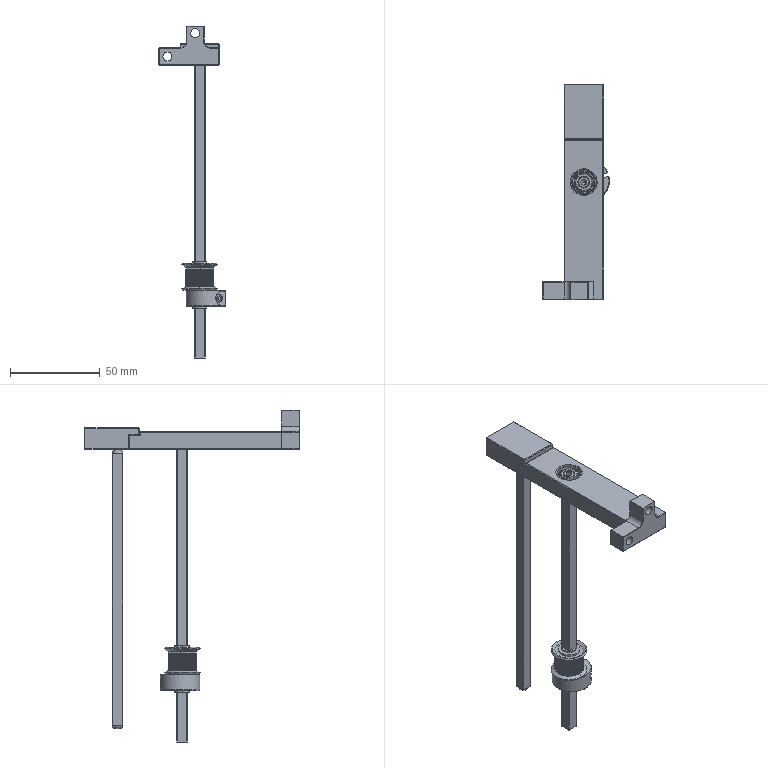Part | NX | features BREP 8 | 8 solids | 619 faces | box 37.325 x 120 x 185 mm | volume 44001 mm3 | plane 244 | cylinder 233 | sphere 64 | cone 42 | torus 36 | commonest cylinder face diameters 0.46 x120 15.66 x25 8 x8 3.4 x7 3.3 x6 6 x6